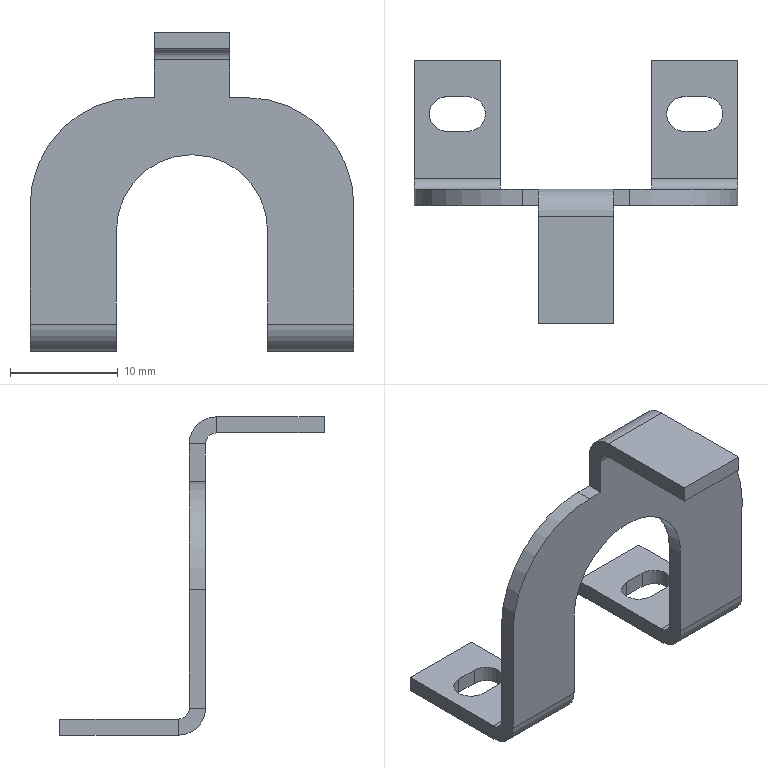Part | SolidWorks | features Fillet 3, ICE 3, EdgeFlange 2, Cut 1, FlatPattern 1, SMBaseFlange 1, SheetMetal 1 | 1 solid | 51 faces | box 30 x 24.5 x 29.5 mm | volume 1040 mm3 | plane 35 | cylinder 16 | commonest cylinder face diameters 3.2 x6 2 x3 5 x3 14 x2 20 x2
STEP:
#1=CARTESIAN_POINT('',(-1.685,53.528,-1.5));
#2=VERTEX_POINT('',#1);
#3=CARTESIAN_POINT('',(-0.08512,51.928,-1.5));
#4=VERTEX_POINT('',#3);
#5=CARTESIAN_POINT('',(-1.685,51.928,-1.5));
#6=DIRECTION('',(0.,0.,-1.));
#7=DIRECTION('',(-1.,0.,0.));
#8=AXIS2_PLACEMENT_3D('',#5,#6,#7);
#9=CIRCLE('',#8,1.6);
#10=EDGE_CURVE('',#2,#4,#9,.T.);
#11=ORIENTED_EDGE('',*,*,#10,.T.);
#12=CARTESIAN_POINT('',(-0.08512,51.928,0.));
#13=VERTEX_POINT('',#12);
#14=CARTESIAN_POINT('',(-0.08512,51.928,-10.));
#15=DIRECTION('',(0.,0.,1.));
#16=VECTOR('',#15,1000.);
#17=LINE('',#14,#16);
#18=EDGE_CURVE('',#4,#13,#17,.T.);
#19=ORIENTED_EDGE('',*,*,#18,.T.);
#20=CARTESIAN_POINT('',(-1.685,53.528,0.));
#21=VERTEX_POINT('',#20);
#22=CARTESIAN_POINT('',(-1.685,51.928,0.));
#23=DIRECTION('',(0.,0.,1.));
#24=DIRECTION('',(1.,0.,0.));
#25=AXIS2_PLACEMENT_3D('',#22,#23,#24);
#26=CIRCLE('',#25,1.6);
#27=EDGE_CURVE('',#13,#21,#26,.T.);
#28=ORIENTED_EDGE('',*,*,#27,.T.);
#29=CARTESIAN_POINT('',(-1.685,53.528,-10.));
#30=DIRECTION('',(0.,0.,1.));
#31=VECTOR('',#30,1000.);
#32=LINE('',#29,#31);
#33=EDGE_CURVE('',#2,#21,#32,.T.);
#34=ORIENTED_EDGE('',*,*,#33,.F.);
#35=EDGE_LOOP('',(#11,#19,#28,#34));
#36=FACE_OUTER_BOUND('',#35,.T.);
#37=CARTESIAN_POINT('',(-1.685,51.928,-10.));
#38=DIRECTION('',(0.,0.,1.));
#39=DIRECTION('',(1.,0.,0.));
#40=AXIS2_PLACEMENT_3D('',#37,#38,#39);
#41=CYLINDRICAL_SURFACE('',#40,1.6);
#42=ADVANCED_FACE('',(#36),#41,.F.);
#43=CARTESIAN_POINT('',(-23.685,53.528,-1.5));
#44=VERTEX_POINT('',#43);
#45=CARTESIAN_POINT('',(-22.085,51.928,-1.5));
#46=VERTEX_POINT('',#45);
#47=CARTESIAN_POINT('',(-23.685,51.928,-1.5));
#48=DIRECTION('',(0.,0.,-1.));
#49=DIRECTION('',(-1.,0.,0.));
#50=AXIS2_PLACEMENT_3D('',#47,#48,#49);
#51=CIRCLE('',#50,1.6);
#52=EDGE_CURVE('',#44,#46,#51,.T.);
#53=ORIENTED_EDGE('',*,*,#52,.T.);
#54=CARTESIAN_POINT('',(-22.085,51.928,0.));
#55=VERTEX_POINT('',#54);
#56=CARTESIAN_POINT('',(-22.085,51.928,-10.));
#57=DIRECTION('',(0.,0.,1.));
#58=VECTOR('',#57,1000.);
#59=LINE('',#56,#58);
#60=EDGE_CURVE('',#46,#55,#59,.T.);
#61=ORIENTED_EDGE('',*,*,#60,.T.);
#62=CARTESIAN_POINT('',(-23.685,53.528,0.));
#63=VERTEX_POINT('',#62);
#64=CARTESIAN_POINT('',(-23.685,51.928,0.));
#65=DIRECTION('',(0.,0.,1.));
#66=DIRECTION('',(1.,0.,0.));
#67=AXIS2_PLACEMENT_3D('',#64,#65,#66);
#68=CIRCLE('',#67,1.6);
#69=EDGE_CURVE('',#55,#63,#68,.T.);
#70=ORIENTED_EDGE('',*,*,#69,.T.);
#71=CARTESIAN_POINT('',(-23.685,53.528,-10.));
#72=DIRECTION('',(0.,0.,1.));
#73=VECTOR('',#72,1000.);
#74=LINE('',#71,#73);
#75=EDGE_CURVE('',#44,#63,#74,.T.);
#76=ORIENTED_EDGE('',*,*,#75,.F.);
#77=EDGE_LOOP('',(#53,#61,#70,#76));
#78=FACE_OUTER_BOUND('',#77,.T.);
#79=CARTESIAN_POINT('',(-23.685,51.928,-10.));
#80=DIRECTION('',(0.,0.,1.));
#81=DIRECTION('',(1.,0.,0.));
#82=AXIS2_PLACEMENT_3D('',#79,#80,#81);
#83=CYLINDRICAL_SURFACE('',#82,1.6);
#84=ADVANCED_FACE('',(#78),#83,.F.);
#85=CARTESIAN_POINT('',(-6.685,56.928,-1.5));
#86=VERTEX_POINT('',#85);
#87=CARTESIAN_POINT('',(-6.685,45.928,-1.5));
#88=VERTEX_POINT('',#87);
#89=CARTESIAN_POINT('',(-6.685,0.,-1.5));
#90=DIRECTION('',(0.,-1.,0.));
#91=VECTOR('',#90,1000.);
#92=LINE('',#89,#91);
#93=EDGE_CURVE('',#86,#88,#92,.T.);
#94=ORIENTED_EDGE('',*,*,#93,.T.);
#95=CARTESIAN_POINT('',(-6.685,45.928,0.));
#96=VERTEX_POINT('',#95);
#97=CARTESIAN_POINT('',(-6.685,45.928,-1.5));
#98=DIRECTION('',(0.,0.,1.));
#99=VECTOR('',#98,1000.);
#100=LINE('',#97,#99);
#101=EDGE_CURVE('',#88,#96,#100,.T.);
#102=ORIENTED_EDGE('',*,*,#101,.T.);
#103=CARTESIAN_POINT('',(-6.685,56.928,0.));
#104=VERTEX_POINT('',#103);
#105=CARTESIAN_POINT('',(-6.685,0.,0.));
#106=DIRECTION('',(0.,-1.,0.));
#107=VECTOR('',#106,1000.);
#108=LINE('',#105,#107);
#109=EDGE_CURVE('',#104,#96,#108,.T.);
#110=ORIENTED_EDGE('',*,*,#109,.F.);
#111=CARTESIAN_POINT('',(-6.685,56.928,-3.296));
#112=DIRECTION('',(0.,0.,-1.));
#113=VECTOR('',#112,1000.);
#114=LINE('',#111,#113);
#115=EDGE_CURVE('',#104,#86,#114,.T.);
#116=ORIENTED_EDGE('',*,*,#115,.T.);
#117=EDGE_LOOP('',(#94,#102,#110,#116));
#118=FACE_OUTER_BOUND('',#117,.T.);
#119=CARTESIAN_POINT('',(-6.685,32.427,-3.296));
#120=DIRECTION('',(1.,0.,0.));
#121=DIRECTION('',(0.,0.,-1.));
#122=AXIS2_PLACEMENT_3D('',#119,#120,#121);
#123=PLANE('',#122);
#124=ADVANCED_FACE('',(#118),#123,.F.);
#125=CARTESIAN_POINT('',(-6.685,43.428,9.704));
#126=VERTEX_POINT('',#125);
#127=CARTESIAN_POINT('',(-6.685,43.428,1.));
#128=VERTEX_POINT('',#127);
#129=CARTESIAN_POINT('',(-6.685,43.428,0.));
#130=DIRECTION('',(0.,0.,-1.));
#131=VECTOR('',#130,1000.);
#132=LINE('',#129,#131);
#133=EDGE_CURVE('',#126,#128,#132,.T.);
#134=ORIENTED_EDGE('',*,*,#133,.F.);
#135=CARTESIAN_POINT('',(-6.685,44.928,9.704));
#136=VERTEX_POINT('',#135);
#137=CARTESIAN_POINT('',(-6.685,44.928,9.704));
#138=DIRECTION('',(0.,1.,0.));
#139=VECTOR('',#138,1000.);
#140=LINE('',#137,#139);
#141=EDGE_CURVE('',#126,#136,#140,.T.);
#142=ORIENTED_EDGE('',*,*,#141,.T.);
#143=CARTESIAN_POINT('',(-6.685,44.928,1.));
#144=VERTEX_POINT('',#143);
#145=CARTESIAN_POINT('',(-6.685,44.928,0.));
#146=DIRECTION('',(0.,0.,-1.));
#147=VECTOR('',#146,1000.);
#148=LINE('',#145,#147);
#149=EDGE_CURVE('',#136,#144,#148,.T.);
#150=ORIENTED_EDGE('',*,*,#149,.T.);
#151=CARTESIAN_POINT('',(-6.685,44.928,1.));
#152=DIRECTION('',(0.,-1.,0.));
#153=VECTOR('',#152,1000.);
#154=LINE('',#151,#153);
#155=EDGE_CURVE('',#144,#128,#154,.T.);
#156=ORIENTED_EDGE('',*,*,#155,.T.);
#157=EDGE_LOOP('',(#134,#142,#150,#156));
#158=FACE_OUTER_BOUND('',#157,.T.);
#159=CARTESIAN_POINT('',(-6.685,32.427,-3.296));
#160=DIRECTION('',(1.,0.,0.));
#161=DIRECTION('',(0.,0.,-1.));
#162=AXIS2_PLACEMENT_3D('',#159,#160,#161);
#163=PLANE('',#162);
#164=ADVANCED_FACE('',(#158),#163,.F.);
#165=CARTESIAN_POINT('',(-20.685,45.928,0.));
#166=VERTEX_POINT('',#165);
#167=CARTESIAN_POINT('',(-20.685,56.928,0.));
#168=VERTEX_POINT('',#167);
#169=CARTESIAN_POINT('',(-20.685,0.,0.));
#170=DIRECTION('',(0.,1.,0.));
#171=VECTOR('',#170,1000.);
#172=LINE('',#169,#171);
#173=EDGE_CURVE('',#166,#168,#172,.T.);
#174=ORIENTED_EDGE('',*,*,#173,.F.);
#175=CARTESIAN_POINT('',(-20.685,45.928,-1.5));
#176=VERTEX_POINT('',#175);
#177=CARTESIAN_POINT('',(-20.685,45.928,0.));
#178=DIRECTION('',(0.,0.,-1.));
#179=VECTOR('',#178,1000.);
#180=LINE('',#177,#179);
#181=EDGE_CURVE('',#166,#176,#180,.T.);
#182=ORIENTED_EDGE('',*,*,#181,.T.);
#183=CARTESIAN_POINT('',(-20.685,56.928,-1.5));
#184=VERTEX_POINT('',#183);
#185=CARTESIAN_POINT('',(-20.685,0.,-1.5));
#186=DIRECTION('',(0.,1.,0.));
#187=VECTOR('',#186,1000.);
#188=LINE('',#185,#187);
#189=EDGE_CURVE('',#176,#184,#188,.T.);
#190=ORIENTED_EDGE('',*,*,#189,.T.);
#191=CARTESIAN_POINT('',(-20.685,56.928,-3.296));
#192=DIRECTION('',(0.,0.,1.));
#193=VECTOR('',#192,1000.);
#194=LINE('',#191,#193);
#195=EDGE_CURVE('',#184,#168,#194,.T.);
#196=ORIENTED_EDGE('',*,*,#195,.T.);
#197=EDGE_LOOP('',(#174,#182,#190,#196));
#198=FACE_OUTER_BOUND('',#197,.T.);
#199=CARTESIAN_POINT('',(-20.685,32.427,-3.296));
#200=DIRECTION('',(-1.,0.,0.));
#201=DIRECTION('',(0.,0.,1.));
#202=AXIS2_PLACEMENT_3D('',#199,#200,#201);
#203=PLANE('',#202);
#204=ADVANCED_FACE('',(#198),#203,.F.);
#205=CARTESIAN_POINT('',(-20.685,44.928,1.));
#206=VERTEX_POINT('',#205);
#207=CARTESIAN_POINT('',(-20.685,44.928,9.704));
#208=VERTEX_POINT('',#207);
#209=CARTESIAN_POINT('',(-20.685,44.928,0.));
#210=DIRECTION('',(0.,0.,1.));
#211=VECTOR('',#210,1000.);
#212=LINE('',#209,#211);
#213=EDGE_CURVE('',#206,#208,#212,.T.);
#214=ORIENTED_EDGE('',*,*,#213,.T.);
#215=CARTESIAN_POINT('',(-20.685,43.428,9.704));
#216=VERTEX_POINT('',#215);
#217=CARTESIAN_POINT('',(-20.685,43.428,9.704));
#218=DIRECTION('',(0.,-1.,0.));
#219=VECTOR('',#218,1000.);
#220=LINE('',#217,#219);
#221=EDGE_CURVE('',#208,#216,#220,.T.);
#222=ORIENTED_EDGE('',*,*,#221,.T.);
#223=CARTESIAN_POINT('',(-20.685,43.428,1.));
#224=VERTEX_POINT('',#223);
#225=CARTESIAN_POINT('',(-20.685,43.428,0.));
#226=DIRECTION('',(0.,0.,1.));
#227=VECTOR('',#226,1000.);
#228=LINE('',#225,#227);
#229=EDGE_CURVE('',#224,#216,#228,.T.);
#230=ORIENTED_EDGE('',*,*,#229,.F.);
#231=CARTESIAN_POINT('',(-20.685,43.428,1.));
#232=DIRECTION('',(0.,1.,0.));
#233=VECTOR('',#232,1000.);
#234=LINE('',#231,#233);
#235=EDGE_CURVE('',#224,#206,#234,.T.);
#236=ORIENTED_EDGE('',*,*,#235,.T.);
#237=EDGE_LOOP('',(#214,#222,#230,#236));
#238=FACE_OUTER_BOUND('',#237,.T.);
#239=CARTESIAN_POINT('',(-20.685,32.427,-3.296));
#240=DIRECTION('',(-1.,0.,0.));
#241=DIRECTION('',(0.,0.,1.));
#242=AXIS2_PLACEMENT_3D('',#239,#240,#241);
#243=PLANE('',#242);
#244=ADVANCED_FACE('',(#238),#243,.F.);
#245=CARTESIAN_POINT('',(-25.685,50.328,-1.5));
#246=VERTEX_POINT('',#245);
#247=CARTESIAN_POINT('',(-25.685,53.528,-1.5));
#248=VERTEX_POINT('',#247);
#249=CARTESIAN_POINT('',(-25.685,51.928,-1.5));
#250=DIRECTION('',(0.,0.,-1.));
#251=DIRECTION('',(-1.,0.,0.));
#252=AXIS2_PLACEMENT_3D('',#249,#250,#251);
#253=CIRCLE('',#252,1.6);
#254=EDGE_CURVE('',#246,#248,#253,.T.);
#255=ORIENTED_EDGE('',*,*,#254,.F.);
#256=CARTESIAN_POINT('',(-23.685,50.328,-1.5));
#257=VERTEX_POINT('',#256);
#258=CARTESIAN_POINT('',(0.,50.328,-1.5));
#259=DIRECTION('',(-1.,0.,0.));
#260=VECTOR('',#259,1000.);
#261=LINE('',#258,#260);
#262=EDGE_CURVE('',#257,#246,#261,.T.);
#263=ORIENTED_EDGE('',*,*,#262,.F.);
#264=CARTESIAN_POINT('',(-23.685,51.928,-1.5));
#265=DIRECTION('',(0.,0.,-1.));
#266=DIRECTION('',(-1.,0.,0.));
#267=AXIS2_PLACEMENT_3D('',#264,#265,#266);
#268=CIRCLE('',#267,1.6);
#269=EDGE_CURVE('',#46,#257,#268,.T.);
#270=ORIENTED_EDGE('',*,*,#269,.F.);
#271=ORIENTED_EDGE('',*,*,#52,.F.);
#272=CARTESIAN_POINT('',(0.,53.528,-1.5));
#273=DIRECTION('',(1.,0.,0.));
#274=VECTOR('',#273,1000.);
#275=LINE('',#272,#274);
#276=EDGE_CURVE('',#248,#44,#275,.T.);
#277=ORIENTED_EDGE('',*,*,#276,.F.);
#278=EDGE_LOOP('',(#255,#263,#270,#271,#277));
#279=FACE_BOUND('',#278,.T.);
#280=ORIENTED_EDGE('',*,*,#189,.F.);
#281=CARTESIAN_POINT('',(-28.685,45.928,-1.5));
#282=VERTEX_POINT('',#281);
#283=CARTESIAN_POINT('',(1.315,45.928,-1.5));
#284=DIRECTION('',(-1.,0.,0.));
#285=VECTOR('',#284,1000.);
#286=LINE('',#283,#285);
#287=EDGE_CURVE('',#176,#282,#286,.T.);
#288=ORIENTED_EDGE('',*,*,#287,.T.);
#289=CARTESIAN_POINT('',(-28.685,56.928,-1.5));
#290=VERTEX_POINT('',#289);
#291=CARTESIAN_POINT('',(-28.685,56.928,-1.5));
#292=DIRECTION('',(0.,-1.,0.));
#293=VECTOR('',#292,1000.);
#294=LINE('',#291,#293);
#295=EDGE_CURVE('',#290,#282,#294,.T.);
#296=ORIENTED_EDGE('',*,*,#295,.F.);
#297=CARTESIAN_POINT('',(1.315,56.928,-1.5));
#298=DIRECTION('',(-1.,0.,0.));
#299=VECTOR('',#298,1000.);
#300=LINE('',#297,#299);
#301=EDGE_CURVE('',#184,#290,#300,.T.);
#302=ORIENTED_EDGE('',*,*,#301,.F.);
#303=EDGE_LOOP('',(#280,#288,#296,#302));
#304=FACE_OUTER_BOUND('',#303,.T.);
#305=CARTESIAN_POINT('',(0.,0.,-1.5));
#306=DIRECTION('',(0.,0.,-1.));
#307=DIRECTION('',(-1.,0.,0.));
#308=AXIS2_PLACEMENT_3D('',#305,#306,#307);
#309=PLANE('',#308);
#310=ADVANCED_FACE('',(#279,#304),#309,.T.);
#311=CARTESIAN_POINT('',(-25.685,50.328,0.));
#312=VERTEX_POINT('',#311);
#313=CARTESIAN_POINT('',(-23.685,50.328,0.));
#314=VERTEX_POINT('',#313);
#315=CARTESIAN_POINT('',(-25.685,50.328,0.));
#316=DIRECTION('',(1.,0.,0.));
#317=VECTOR('',#316,1000.);
#318=LINE('',#315,#317);
#319=EDGE_CURVE('',#312,#314,#318,.T.);
#320=ORIENTED_EDGE('',*,*,#319,.F.);
#321=CARTESIAN_POINT('',(-25.685,53.528,0.));
#322=VERTEX_POINT('',#321);
#323=CARTESIAN_POINT('',(-25.685,51.928,0.));
#324=DIRECTION('',(0.,0.,1.));
#325=DIRECTION('',(1.,0.,0.));
#326=AXIS2_PLACEMENT_3D('',#323,#324,#325);
#327=CIRCLE('',#326,1.6);
#328=EDGE_CURVE('',#322,#312,#327,.T.);
#329=ORIENTED_EDGE('',*,*,#328,.F.);
#330=CARTESIAN_POINT('',(-25.685,53.528,0.));
#331=DIRECTION('',(-1.,0.,0.));
#332=VECTOR('',#331,1000.);
#333=LINE('',#330,#332);
#334=EDGE_CURVE('',#63,#322,#333,.T.);
#335=ORIENTED_EDGE('',*,*,#334,.F.);
#336=ORIENTED_EDGE('',*,*,#69,.F.);
#337=CARTESIAN_POINT('',(-23.685,51.928,0.));
#338=DIRECTION('',(0.,0.,1.));
#339=DIRECTION('',(1.,0.,0.));
#340=AXIS2_PLACEMENT_3D('',#337,#338,#339);
#341=CIRCLE('',#340,1.6);
#342=EDGE_CURVE('',#314,#55,#341,.T.);
#343=ORIENTED_EDGE('',*,*,#342,.F.);
#344=EDGE_LOOP('',(#320,#329,#335,#336,#343));
#345=FACE_BOUND('',#344,.T.);
#346=CARTESIAN_POINT('',(-28.685,45.928,0.));
#347=VERTEX_POINT('',#346);
#348=CARTESIAN_POINT('',(1.315,45.928,0.));
#349=DIRECTION('',(-1.,0.,0.));
#350=VECTOR('',#349,1000.);
#351=LINE('',#348,#350);
#352=EDGE_CURVE('',#166,#347,#351,.T.);
#353=ORIENTED_EDGE('',*,*,#352,.F.);
#354=ORIENTED_EDGE('',*,*,#173,.T.);
#355=CARTESIAN_POINT('',(-28.685,56.928,0.));
#356=VERTEX_POINT('',#355);
#357=CARTESIAN_POINT('',(1.315,56.928,0.));
#358=DIRECTION('',(-1.,0.,0.));
#359=VECTOR('',#358,1000.);
#360=LINE('',#357,#359);
#361=EDGE_CURVE('',#168,#356,#360,.T.);
#362=ORIENTED_EDGE('',*,*,#361,.T.);
#363=CARTESIAN_POINT('',(-28.685,56.928,0.));
#364=DIRECTION('',(0.,-1.,0.));
#365=VECTOR('',#364,1000.);
#366=LINE('',#363,#365);
#367=EDGE_CURVE('',#356,#347,#366,.T.);
#368=ORIENTED_EDGE('',*,*,#367,.T.);
#369=EDGE_LOOP('',(#353,#354,#362,#368));
#370=FACE_OUTER_BOUND('',#369,.T.);
#371=CARTESIAN_POINT('',(0.,0.,0.));
#372=DIRECTION('',(0.,0.,-1.));
#373=DIRECTION('',(-1.,0.,0.));
#374=AXIS2_PLACEMENT_3D('',#371,#372,#373);
#375=PLANE('',#374);
#376=ADVANCED_FACE('',(#345,#370),#375,.F.);
#377=ORIENTED_EDGE('',*,*,#195,.F.);
#378=ORIENTED_EDGE('',*,*,#301,.T.);
#379=CARTESIAN_POINT('',(-28.685,56.928,-1.5));
#380=DIRECTION('',(0.,0.,1.));
#381=VECTOR('',#380,1000.);
#382=LINE('',#379,#381);
#383=EDGE_CURVE('',#290,#356,#382,.T.);
#384=ORIENTED_EDGE('',*,*,#383,.T.);
#385=ORIENTED_EDGE('',*,*,#361,.F.);
#386=EDGE_LOOP('',(#377,#378,#384,#385));
#387=FACE_OUTER_BOUND('',#386,.T.);
#388=CARTESIAN_POINT('',(1.315,56.928,-1.5));
#389=DIRECTION('',(0.,1.,0.));
#390=DIRECTION('',(0.,0.,1.));
#391=AXIS2_PLACEMENT_3D('',#388,#389,#390);
#392=PLANE('',#391);
#393=ADVANCED_FACE('',(#387),#392,.T.);
#394=CARTESIAN_POINT('',(-20.685,45.928,1.));
#395=DIRECTION('',(1.,0.,0.));
#396=DIRECTION('',(0.,0.,1.));
#397=AXIS2_PLACEMENT_3D('',#394,#395,#396);
#398=CIRCLE('',#397,2.5);
#399=EDGE_CURVE('',#224,#176,#398,.T.);
#400=ORIENTED_EDGE('',*,*,#399,.F.);
#401=CARTESIAN_POINT('',(-28.685,43.428,1.));
#402=VERTEX_POINT('',#401);
#403=CARTESIAN_POINT('',(0.,43.428,1.));
#404=DIRECTION('',(-1.,0.,0.));
#405=VECTOR('',#404,1000.);
#406=LINE('',#403,#405);
#407=EDGE_CURVE('',#224,#402,#406,.T.);
#408=ORIENTED_EDGE('',*,*,#407,.T.);
#409=CARTESIAN_POINT('',(-28.685,45.928,1.));
#410=DIRECTION('',(-1.,0.,0.));
#411=DIRECTION('',(0.,0.,-1.));
#412=AXIS2_PLACEMENT_3D('',#409,#410,#411);
#413=CIRCLE('',#412,2.5);
#414=EDGE_CURVE('',#282,#402,#413,.T.);
#415=ORIENTED_EDGE('',*,*,#414,.F.);
#416=ORIENTED_EDGE('',*,*,#287,.F.);
#417=EDGE_LOOP('',(#400,#408,#415,#416));
#418=FACE_OUTER_BOUND('',#417,.T.);
#419=CARTESIAN_POINT('',(1.315,45.928,1.));
#420=DIRECTION('',(1.,0.,0.));
#421=DIRECTION('',(0.,-1.,0.));
#422=AXIS2_PLACEMENT_3D('',#419,#420,#421);
#423=CYLINDRICAL_SURFACE('',#422,2.5);
#424=ADVANCED_FACE('',(#418),#423,.T.);
#425=CARTESIAN_POINT('',(-28.685,44.928,1.));
#426=VERTEX_POINT('',#425);
#427=CARTESIAN_POINT('',(-28.685,44.928,1.));
#428=DIRECTION('',(1.,0.,0.));
#429=VECTOR('',#428,1000.);
#430=LINE('',#427,#429);
#431=EDGE_CURVE('',#426,#206,#430,.T.);
#432=ORIENTED_EDGE('',*,*,#431,.T.);
#433=CARTESIAN_POINT('',(-20.685,45.928,1.));
#434=DIRECTION('',(1.,0.,0.));
#435=DIRECTION('',(0.,0.,1.));
#436=AXIS2_PLACEMENT_3D('',#433,#434,#435);
#437=CIRCLE('',#436,1.);
#438=EDGE_CURVE('',#206,#166,#437,.T.);
#439=ORIENTED_EDGE('',*,*,#438,.T.);
#440=ORIENTED_EDGE('',*,*,#352,.T.);
#441=CARTESIAN_POINT('',(-28.685,45.928,1.));
#442=DIRECTION('',(-1.,0.,0.));
#443=DIRECTION('',(0.,0.,-1.));
#444=AXIS2_PLACEMENT_3D('',#441,#442,#443);
#445=CIRCLE('',#444,1.);
#446=EDGE_CURVE('',#347,#426,#445,.T.);
#447=ORIENTED_EDGE('',*,*,#446,.T.);
#448=EDGE_LOOP('',(#432,#439,#440,#447));
#449=FACE_OUTER_BOUND('',#448,.T.);
#450=CARTESIAN_POINT('',(1.315,45.928,1.));
#451=DIRECTION('',(1.,0.,0.));
#452=DIRECTION('',(0.,-1.,0.));
#453=AXIS2_PLACEMENT_3D('',#450,#451,#452);
#454=CYLINDRICAL_SURFACE('',#453,1.);
#455=ADVANCED_FACE('',(#449),#454,.F.);
#456=CARTESIAN_POINT('',(1.315,43.428,1.));
#457=VERTEX_POINT('',#456);
#458=CARTESIAN_POINT('',(1.315,43.428,12.));
#459=VERTEX_POINT('',#458);
#460=CARTESIAN_POINT('',(1.315,43.427,26.5));
#461=DIRECTION('',(0.,0.,1.));
#462=VECTOR('',#461,1000.);
#463=LINE('',#460,#462);
#464=EDGE_CURVE('',#457,#459,#463,.T.);
#465=ORIENTED_EDGE('',*,*,#464,.T.);
#466=CARTESIAN_POINT('',(-8.685,43.428,22.));
#467=VERTEX_POINT('',#466);
#468=CARTESIAN_POINT('',(-8.685,43.428,12.));
#469=DIRECTION('',(0.,-1.,0.));
#470=DIRECTION('',(0.,0.,1.));
#471=AXIS2_PLACEMENT_3D('',#468,#469,#470);
#472=CIRCLE('',#471,10.);
#473=EDGE_CURVE('',#459,#467,#472,.T.);
#474=ORIENTED_EDGE('',*,*,#473,.T.);
#475=CARTESIAN_POINT('',(-10.185,43.428,22.));
#476=VERTEX_POINT('',#475);
#477=CARTESIAN_POINT('',(0.,43.428,22.));
#478=DIRECTION('',(1.,0.,0.));
#479=VECTOR('',#478,1000.);
#480=LINE('',#477,#479);
#481=EDGE_CURVE('',#476,#467,#480,.T.);
#482=ORIENTED_EDGE('',*,*,#481,.F.);
#483=CARTESIAN_POINT('',(-10.185,43.427,25.5));
#484=VERTEX_POINT('',#483);
#485=CARTESIAN_POINT('',(-10.185,43.428,0.));
#486=DIRECTION('',(0.,0.,1.));
#487=VECTOR('',#486,1000.);
#488=LINE('',#485,#487);
#489=EDGE_CURVE('',#476,#484,#488,.T.);
#490=ORIENTED_EDGE('',*,*,#489,.T.);
#491=CARTESIAN_POINT('',(-17.185,43.427,25.5));
#492=VERTEX_POINT('',#491);
#493=CARTESIAN_POINT('',(-28.685,43.427,25.5));
#494=DIRECTION('',(1.,0.,0.));
#495=VECTOR('',#494,1000.);
#496=LINE('',#493,#495);
#497=EDGE_CURVE('',#492,#484,#496,.T.);
#498=ORIENTED_EDGE('',*,*,#497,.F.);
#499=CARTESIAN_POINT('',(-17.185,43.427,22.));
#500=VERTEX_POINT('',#499);
#501=CARTESIAN_POINT('',(-17.185,43.428,0.));
#502=DIRECTION('',(0.,0.,-1.));
#503=VECTOR('',#502,1000.);
#504=LINE('',#501,#503);
#505=EDGE_CURVE('',#492,#500,#504,.T.);
#506=ORIENTED_EDGE('',*,*,#505,.T.);
#507=CARTESIAN_POINT('',(-18.685,43.427,22.));
#508=VERTEX_POINT('',#507);
#509=CARTESIAN_POINT('',(0.,43.428,22.));
#510=DIRECTION('',(-1.,0.,0.));
#511=VECTOR('',#510,1000.);
#512=LINE('',#509,#511);
#513=EDGE_CURVE('',#500,#508,#512,.T.);
#514=ORIENTED_EDGE('',*,*,#513,.T.);
#515=CARTESIAN_POINT('',(-28.685,43.428,12.));
#516=VERTEX_POINT('',#515);
#517=CARTESIAN_POINT('',(-18.685,43.428,12.));
#518=DIRECTION('',(0.,-1.,0.));
#519=DIRECTION('',(0.,0.,1.));
#520=AXIS2_PLACEMENT_3D('',#517,#518,#519);
#521=CIRCLE('',#520,10.);
#522=EDGE_CURVE('',#508,#516,#521,.T.);
#523=ORIENTED_EDGE('',*,*,#522,.T.);
#524=CARTESIAN_POINT('',(-28.685,43.428,0.));
#525=DIRECTION('',(0.,0.,-1.));
#526=VECTOR('',#525,1000.);
#527=LINE('',#524,#526);
#528=EDGE_CURVE('',#516,#402,#527,.T.);
#529=ORIENTED_EDGE('',*,*,#528,.T.);
#530=ORIENTED_EDGE('',*,*,#407,.F.);
#531=ORIENTED_EDGE('',*,*,#229,.T.);
#532=CARTESIAN_POINT('',(-13.685,43.428,16.704));
#533=VERTEX_POINT('',#532);
#534=CARTESIAN_POINT('',(-13.685,43.428,9.704));
#535=DIRECTION('',(0.,1.,0.));
#536=DIRECTION('',(0.,0.,1.));
#537=AXIS2_PLACEMENT_3D('',#534,#535,#536);
#538=CIRCLE('',#537,7.);
#539=EDGE_CURVE('',#216,#533,#538,.T.);
#540=ORIENTED_EDGE('',*,*,#539,.T.);
#541=CARTESIAN_POINT('',(-13.685,43.428,9.704));
#542=DIRECTION('',(0.,1.,0.));
#543=DIRECTION('',(0.,0.,1.));
#544=AXIS2_PLACEMENT_3D('',#541,#542,#543);
#545=CIRCLE('',#544,7.);
#546=EDGE_CURVE('',#533,#126,#545,.T.);
#547=ORIENTED_EDGE('',*,*,#546,.T.);
#548=ORIENTED_EDGE('',*,*,#133,.T.);
#549=CARTESIAN_POINT('',(0.,43.428,1.));
#550=DIRECTION('',(-1.,0.,0.));
#551=VECTOR('',#550,1000.);
#552=LINE('',#549,#551);
#553=EDGE_CURVE('',#457,#128,#552,.T.);
#554=ORIENTED_EDGE('',*,*,#553,.F.);
#555=EDGE_LOOP('',(#465,#474,#482,#490,#498,#506,#514,#523,#529,#530,#531,#540,#547,#548,#554));
#556=FACE_OUTER_BOUND('',#555,.T.);
#557=CARTESIAN_POINT('',(0.,43.428,0.));
#558=DIRECTION('',(0.,1.,0.));
#559=DIRECTION('',(0.,0.,1.));
#560=AXIS2_PLACEMENT_3D('',#557,#558,#559);
#561=PLANE('',#560);
#562=ADVANCED_FACE('',(#556),#561,.F.);
#563=CARTESIAN_POINT('',(-10.185,44.928,22.));
#564=VERTEX_POINT('',#563);
#565=CARTESIAN_POINT('',(-8.685,44.928,22.));
#566=VERTEX_POINT('',#565);
#567=CARTESIAN_POINT('',(0.,44.928,22.));
#568=DIRECTION('',(1.,0.,0.));
#569=VECTOR('',#568,1000.);
#570=LINE('',#567,#569);
#571=EDGE_CURVE('',#564,#566,#570,.T.);
#572=ORIENTED_EDGE('',*,*,#571,.T.);
#573=CARTESIAN_POINT('',(1.315,44.928,12.));
#574=VERTEX_POINT('',#573);
#575=CARTESIAN_POINT('',(-8.685,44.928,12.));
#576=DIRECTION('',(0.,1.,0.));
#577=DIRECTION('',(0.,0.,1.));
#578=AXIS2_PLACEMENT_3D('',#575,#576,#577);
#579=CIRCLE('',#578,10.);
#580=EDGE_CURVE('',#566,#574,#579,.T.);
#581=ORIENTED_EDGE('',*,*,#580,.T.);
#582=CARTESIAN_POINT('',(1.315,44.928,1.));
#583=VERTEX_POINT('',#582);
#584=CARTESIAN_POINT('',(1.315,44.927,26.5));
#585=DIRECTION('',(0.,0.,1.));
#586=VECTOR('',#585,1000.);
#587=LINE('',#584,#586);
#588=EDGE_CURVE('',#583,#574,#587,.T.);
#589=ORIENTED_EDGE('',*,*,#588,.F.);
#590=CARTESIAN_POINT('',(-28.685,44.928,1.));
#591=DIRECTION('',(1.,0.,0.));
#592=VECTOR('',#591,1000.);
#593=LINE('',#590,#592);
#594=EDGE_CURVE('',#144,#583,#593,.T.);
#595=ORIENTED_EDGE('',*,*,#594,.F.);
#596=ORIENTED_EDGE('',*,*,#149,.F.);
#597=CARTESIAN_POINT('',(-13.685,44.928,16.704));
#598=VERTEX_POINT('',#597);
#599=CARTESIAN_POINT('',(-13.685,44.928,9.704));
#600=DIRECTION('',(0.,-1.,0.));
#601=DIRECTION('',(0.,0.,1.));
#602=AXIS2_PLACEMENT_3D('',#599,#600,#601);
#603=CIRCLE('',#602,7.);
#604=EDGE_CURVE('',#136,#598,#603,.T.);
#605=ORIENTED_EDGE('',*,*,#604,.T.);
#606=CARTESIAN_POINT('',(-13.685,44.928,9.704));
#607=DIRECTION('',(0.,-1.,0.));
#608=DIRECTION('',(0.,0.,1.));
#609=AXIS2_PLACEMENT_3D('',#606,#607,#608);
#610=CIRCLE('',#609,7.);
#611=EDGE_CURVE('',#598,#208,#610,.T.);
#612=ORIENTED_EDGE('',*,*,#611,.T.);
#613=ORIENTED_EDGE('',*,*,#213,.F.);
#614=ORIENTED_EDGE('',*,*,#431,.F.);
#615=CARTESIAN_POINT('',(-28.685,44.928,12.));
#616=VERTEX_POINT('',#615);
#617=CARTESIAN_POINT('',(-28.685,44.928,0.));
#618=DIRECTION('',(0.,0.,-1.));
#619=VECTOR('',#618,1000.);
#620=LINE('',#617,#619);
#621=EDGE_CURVE('',#616,#426,#620,.T.);
#622=ORIENTED_EDGE('',*,*,#621,.F.);
#623=CARTESIAN_POINT('',(-18.685,44.927,22.));
#624=VERTEX_POINT('',#623);
#625=CARTESIAN_POINT('',(-18.685,44.928,12.));
#626=DIRECTION('',(0.,1.,0.));
#627=DIRECTION('',(0.,0.,1.));
#628=AXIS2_PLACEMENT_3D('',#625,#626,#627);
#629=CIRCLE('',#628,10.);
#630=EDGE_CURVE('',#616,#624,#629,.T.);
#631=ORIENTED_EDGE('',*,*,#630,.T.);
#632=CARTESIAN_POINT('',(-17.185,44.927,22.));
#633=VERTEX_POINT('',#632);
#634=CARTESIAN_POINT('',(0.,44.928,22.));
#635=DIRECTION('',(-1.,0.,0.));
#636=VECTOR('',#635,1000.);
#637=LINE('',#634,#636);
#638=EDGE_CURVE('',#633,#624,#637,.T.);
#639=ORIENTED_EDGE('',*,*,#638,.F.);
#640=CARTESIAN_POINT('',(-17.185,44.927,25.5));
#641=VERTEX_POINT('',#640);
#642=CARTESIAN_POINT('',(-17.185,44.928,0.));
#643=DIRECTION('',(0.,0.,-1.));
#644=VECTOR('',#643,1000.);
#645=LINE('',#642,#644);
#646=EDGE_CURVE('',#641,#633,#645,.T.);
#647=ORIENTED_EDGE('',*,*,#646,.F.);
#648=CARTESIAN_POINT('',(-10.185,44.927,25.5));
#649=VERTEX_POINT('',#648);
#650=CARTESIAN_POINT('',(-28.685,44.927,25.5));
#651=DIRECTION('',(1.,0.,0.));
#652=VECTOR('',#651,1000.);
#653=LINE('',#650,#652);
#654=EDGE_CURVE('',#641,#649,#653,.T.);
#655=ORIENTED_EDGE('',*,*,#654,.T.);
#656=CARTESIAN_POINT('',(-10.185,44.928,0.));
#657=DIRECTION('',(0.,0.,1.));
#658=VECTOR('',#657,1000.);
#659=LINE('',#656,#658);
#660=EDGE_CURVE('',#564,#649,#659,.T.);
#661=ORIENTED_EDGE('',*,*,#660,.F.);
#662=EDGE_LOOP('',(#572,#581,#589,#595,#596,#605,#612,#613,#614,#622,#631,#639,#647,#655,#661));
#663=FACE_OUTER_BOUND('',#662,.T.);
#664=CARTESIAN_POINT('',(0.,44.928,0.));
#665=DIRECTION('',(0.,1.,0.));
#666=DIRECTION('',(0.,0.,1.));
#667=AXIS2_PLACEMENT_3D('',#664,#665,#666);
#668=PLANE('',#667);
#669=ADVANCED_FACE('',(#663),#668,.T.);
#670=CARTESIAN_POINT('',(-17.185,42.427,28.));
#671=VERTEX_POINT('',#670);
#672=CARTESIAN_POINT('',(-10.185,42.427,28.));
#673=VERTEX_POINT('',#672);
#674=CARTESIAN_POINT('',(0.,42.427,28.));
#675=DIRECTION('',(1.,0.,0.));
#676=VECTOR('',#675,1000.);
#677=LINE('',#674,#676);
#678=EDGE_CURVE('',#671,#673,#677,.T.);
#679=ORIENTED_EDGE('',*,*,#678,.T.);
#680=CARTESIAN_POINT('',(-10.185,42.427,25.5));
#681=DIRECTION('',(1.,0.,0.));
#682=DIRECTION('',(0.,0.,1.));
#683=AXIS2_PLACEMENT_3D('',#680,#681,#682);
#684=CIRCLE('',#683,2.5);
#685=EDGE_CURVE('',#649,#673,#684,.T.);
#686=ORIENTED_EDGE('',*,*,#685,.F.);
#687=ORIENTED_EDGE('',*,*,#654,.F.);
#688=CARTESIAN_POINT('',(-17.185,42.427,25.5));
#689=DIRECTION('',(-1.,0.,0.));
#690=DIRECTION('',(0.,0.,-1.));
#691=AXIS2_PLACEMENT_3D('',#688,#689,#690);
#692=CIRCLE('',#691,2.5);
#693=EDGE_CURVE('',#671,#641,#692,.T.);
#694=ORIENTED_EDGE('',*,*,#693,.F.);
#695=EDGE_LOOP('',(#679,#686,#687,#694));
#696=FACE_OUTER_BOUND('',#695,.T.);
#697=CARTESIAN_POINT('',(-28.685,42.427,25.5));
#698=DIRECTION('',(-1.,0.,0.));
#699=DIRECTION('',(0.,0.,1.));
#700=AXIS2_PLACEMENT_3D('',#697,#698,#699);
#701=CYLINDRICAL_SURFACE('',#700,2.5);
#702=ADVANCED_FACE('',(#696),#701,.T.);
#703=CARTESIAN_POINT('',(-10.185,42.427,26.5));
#704=VERTEX_POINT('',#703);
#705=CARTESIAN_POINT('',(-10.185,42.427,25.5));
#706=DIRECTION('',(1.,0.,0.));
#707=DIRECTION('',(0.,0.,1.));
#708=AXIS2_PLACEMENT_3D('',#705,#706,#707);
#709=CIRCLE('',#708,1.);
#710=EDGE_CURVE('',#484,#704,#709,.T.);
#711=ORIENTED_EDGE('',*,*,#710,.T.);
#712=CARTESIAN_POINT('',(-17.185,42.427,26.5));
#713=VERTEX_POINT('',#712);
#714=CARTESIAN_POINT('',(1.315,42.427,26.5));
#715=DIRECTION('',(-1.,0.,0.));
#716=VECTOR('',#715,1000.);
#717=LINE('',#714,#716);
#718=EDGE_CURVE('',#704,#713,#717,.T.);
#719=ORIENTED_EDGE('',*,*,#718,.T.);
#720=CARTESIAN_POINT('',(-17.185,42.427,25.5));
#721=DIRECTION('',(-1.,0.,0.));
#722=DIRECTION('',(0.,0.,1.));
#723=AXIS2_PLACEMENT_3D('',#720,#721,#722);
#724=CIRCLE('',#723,1.);
#725=EDGE_CURVE('',#713,#492,#724,.T.);
#726=ORIENTED_EDGE('',*,*,#725,.T.);
#727=ORIENTED_EDGE('',*,*,#497,.T.);
#728=EDGE_LOOP('',(#711,#719,#726,#727));
#729=FACE_OUTER_BOUND('',#728,.T.);
#730=CARTESIAN_POINT('',(-28.685,42.427,25.5));
#731=DIRECTION('',(-1.,0.,0.));
#732=DIRECTION('',(0.,0.,1.));
#733=AXIS2_PLACEMENT_3D('',#730,#731,#732);
#734=CYLINDRICAL_SURFACE('',#733,1.);
#735=ADVANCED_FACE('',(#729),#734,.F.);
#736=CARTESIAN_POINT('',(-10.185,32.427,28.));
#737=VERTEX_POINT('',#736);
#738=CARTESIAN_POINT('',(-10.185,0.,28.));
#739=DIRECTION('',(0.,1.,0.));
#740=VECTOR('',#739,1000.);
#741=LINE('',#738,#740);
#742=EDGE_CURVE('',#737,#673,#741,.T.);
#743=ORIENTED_EDGE('',*,*,#742,.T.);
#744=ORIENTED_EDGE('',*,*,#678,.F.);
#745=CARTESIAN_POINT('',(-17.185,32.427,28.));
#746=VERTEX_POINT('',#745);
#747=CARTESIAN_POINT('',(-17.185,32.427,28.));
#748=DIRECTION('',(0.,1.,0.));
#749=VECTOR('',#748,1000.);
#750=LINE('',#747,#749);
#751=EDGE_CURVE('',#746,#671,#750,.T.);
#752=ORIENTED_EDGE('',*,*,#751,.F.);
#753=CARTESIAN_POINT('',(1.315,32.427,28.));
#754=DIRECTION('',(1.,0.,0.));
#755=VECTOR('',#754,1000.);
#756=LINE('',#753,#755);
#757=EDGE_CURVE('',#746,#737,#756,.T.);
#758=ORIENTED_EDGE('',*,*,#757,.T.);
#759=EDGE_LOOP('',(#743,#744,#752,#758));
#760=FACE_OUTER_BOUND('',#759,.T.);
#761=CARTESIAN_POINT('',(0.,0.,28.));
#762=DIRECTION('',(0.,0.,-1.));
#763=DIRECTION('',(-1.,0.,0.));
#764=AXIS2_PLACEMENT_3D('',#761,#762,#763);
#765=PLANE('',#764);
#766=ADVANCED_FACE('',(#760),#765,.F.);
#767=ORIENTED_EDGE('',*,*,#718,.F.);
#768=CARTESIAN_POINT('',(-10.185,32.427,26.5));
#769=VERTEX_POINT('',#768);
#770=CARTESIAN_POINT('',(-10.185,0.,26.5));
#771=DIRECTION('',(0.,1.,0.));
#772=VECTOR('',#771,1000.);
#773=LINE('',#770,#772);
#774=EDGE_CURVE('',#769,#704,#773,.T.);
#775=ORIENTED_EDGE('',*,*,#774,.F.);
#776=CARTESIAN_POINT('',(-17.185,32.427,26.5));
#777=VERTEX_POINT('',#776);
#778=CARTESIAN_POINT('',(1.315,32.427,26.5));
#779=DIRECTION('',(1.,0.,0.));
#780=VECTOR('',#779,1000.);
#781=LINE('',#778,#780);
#782=EDGE_CURVE('',#777,#769,#781,.T.);
#783=ORIENTED_EDGE('',*,*,#782,.F.);
#784=CARTESIAN_POINT('',(-17.185,0.,26.5));
#785=DIRECTION('',(0.,1.,0.));
#786=VECTOR('',#785,1000.);
#787=LINE('',#784,#786);
#788=EDGE_CURVE('',#777,#713,#787,.T.);
#789=ORIENTED_EDGE('',*,*,#788,.T.);
#790=EDGE_LOOP('',(#767,#775,#783,#789));
#791=FACE_OUTER_BOUND('',#790,.T.);
#792=CARTESIAN_POINT('',(0.,0.,26.5));
#793=DIRECTION('',(0.,0.,-1.));
#794=DIRECTION('',(-1.,0.,0.));
#795=AXIS2_PLACEMENT_3D('',#792,#793,#794);
#796=PLANE('',#795);
#797=ADVANCED_FACE('',(#791),#796,.T.);
#798=CARTESIAN_POINT('',(-10.185,32.427,26.5));
#799=DIRECTION('',(0.,0.,1.));
#800=VECTOR('',#799,1000.);
#801=LINE('',#798,#800);
#802=EDGE_CURVE('',#769,#737,#801,.T.);
#803=ORIENTED_EDGE('',*,*,#802,.T.);
#804=ORIENTED_EDGE('',*,*,#757,.F.);
#805=CARTESIAN_POINT('',(-17.185,32.427,28.));
#806=DIRECTION('',(0.,0.,-1.));
#807=VECTOR('',#806,1000.);
#808=LINE('',#805,#807);
#809=EDGE_CURVE('',#746,#777,#808,.T.);
#810=ORIENTED_EDGE('',*,*,#809,.T.);
#811=ORIENTED_EDGE('',*,*,#782,.T.);
#812=EDGE_LOOP('',(#803,#804,#810,#811));
#813=FACE_OUTER_BOUND('',#812,.T.);
#814=CARTESIAN_POINT('',(1.315,32.427,28.));
#815=DIRECTION('',(0.,1.,0.));
#816=DIRECTION('',(0.,0.,1.));
#817=AXIS2_PLACEMENT_3D('',#814,#815,#816);
#818=PLANE('',#817);
#819=ADVANCED_FACE('',(#813),#818,.F.);
#820=ORIENTED_EDGE('',*,*,#588,.T.);
#821=CARTESIAN_POINT('',(1.315,43.428,12.));
#822=DIRECTION('',(0.,-1.,0.));
#823=VECTOR('',#822,1000.);
#824=LINE('',#821,#823);
#825=EDGE_CURVE('',#574,#459,#824,.T.);
#826=ORIENTED_EDGE('',*,*,#825,.T.);
#827=ORIENTED_EDGE('',*,*,#464,.F.);
#828=CARTESIAN_POINT('',(1.315,44.928,1.));
#829=DIRECTION('',(0.,-1.,0.));
#830=VECTOR('',#829,1000.);
#831=LINE('',#828,#830);
#832=EDGE_CURVE('',#583,#457,#831,.T.);
#833=ORIENTED_EDGE('',*,*,#832,.F.);
#834=EDGE_LOOP('',(#820,#826,#827,#833));
#835=FACE_OUTER_BOUND('',#834,.T.);
#836=CARTESIAN_POINT('',(1.315,43.427,26.5));
#837=DIRECTION('',(-1.,0.,0.));
#838=DIRECTION('',(0.,0.,1.));
#839=AXIS2_PLACEMENT_3D('',#836,#837,#838);
#840=PLANE('',#839);
#841=ADVANCED_FACE('',(#835),#840,.F.);
#842=ORIENTED_EDGE('',*,*,#528,.F.);
#843=CARTESIAN_POINT('',(-28.685,44.928,12.));
#844=DIRECTION('',(0.,1.,0.));
#845=VECTOR('',#844,1000.);
#846=LINE('',#843,#845);
#847=EDGE_CURVE('',#516,#616,#846,.T.);
#848=ORIENTED_EDGE('',*,*,#847,.T.);
#849=ORIENTED_EDGE('',*,*,#621,.T.);
#850=CARTESIAN_POINT('',(-28.685,44.928,1.));
#851=DIRECTION('',(0.,-1.,0.));
#852=VECTOR('',#851,1000.);
#853=LINE('',#850,#852);
#854=EDGE_CURVE('',#426,#402,#853,.T.);
#855=ORIENTED_EDGE('',*,*,#854,.T.);
#856=EDGE_LOOP('',(#842,#848,#849,#855));
#857=FACE_OUTER_BOUND('',#856,.T.);
#858=CARTESIAN_POINT('',(-28.685,43.428,0.));
#859=DIRECTION('',(1.,0.,0.));
#860=DIRECTION('',(0.,1.,0.));
#861=AXIS2_PLACEMENT_3D('',#858,#859,#860);
#862=PLANE('',#861);
#863=ADVANCED_FACE('',(#857),#862,.F.);
#864=CARTESIAN_POINT('',(1.315,45.928,0.));
#865=VERTEX_POINT('',#864);
#866=CARTESIAN_POINT('',(1.315,56.928,0.));
#867=VERTEX_POINT('',#866);
#868=CARTESIAN_POINT('',(1.315,56.928,0.));
#869=DIRECTION('',(0.,1.,0.));
#870=VECTOR('',#869,1000.);
#871=LINE('',#868,#870);
#872=EDGE_CURVE('',#865,#867,#871,.T.);
#873=ORIENTED_EDGE('',*,*,#872,.F.);
#874=CARTESIAN_POINT('',(1.315,45.928,-1.5));
#875=VERTEX_POINT('',#874);
#876=CARTESIAN_POINT('',(1.315,45.928,0.));
#877=DIRECTION('',(0.,0.,-1.));
#878=VECTOR('',#877,1000.);
#879=LINE('',#876,#878);
#880=EDGE_CURVE('',#865,#875,#879,.T.);
#881=ORIENTED_EDGE('',*,*,#880,.T.);
#882=CARTESIAN_POINT('',(1.315,56.928,-1.5));
#883=VERTEX_POINT('',#882);
#884=CARTESIAN_POINT('',(1.315,56.928,-1.5));
#885=DIRECTION('',(0.,1.,0.));
#886=VECTOR('',#885,1000.);
#887=LINE('',#884,#886);
#888=EDGE_CURVE('',#875,#883,#887,.T.);
#889=ORIENTED_EDGE('',*,*,#888,.T.);
#890=CARTESIAN_POINT('',(1.315,56.928,-1.5));
#891=DIRECTION('',(0.,0.,1.));
#892=VECTOR('',#891,1000.);
#893=LINE('',#890,#892);
#894=EDGE_CURVE('',#883,#867,#893,.T.);
#895=ORIENTED_EDGE('',*,*,#894,.T.);
#896=EDGE_LOOP('',(#873,#881,#889,#895));
#897=FACE_OUTER_BOUND('',#896,.T.);
#898=CARTESIAN_POINT('',(1.315,56.928,-1.5));
#899=DIRECTION('',(1.,0.,0.));
#900=DIRECTION('',(0.,1.,0.));
#901=AXIS2_PLACEMENT_3D('',#898,#899,#900);
#902=PLANE('',#901);
#903=ADVANCED_FACE('',(#897),#902,.T.);
#904=CARTESIAN_POINT('',(-3.685,50.328,-1.5));
#905=VERTEX_POINT('',#904);
#906=CARTESIAN_POINT('',(-3.685,53.528,-1.5));
#907=VERTEX_POINT('',#906);
#908=CARTESIAN_POINT('',(-3.685,51.928,-1.5));
#909=DIRECTION('',(0.,0.,-1.));
#910=DIRECTION('',(-1.,0.,0.));
#911=AXIS2_PLACEMENT_3D('',#908,#909,#910);
#912=CIRCLE('',#911,1.6);
#913=EDGE_CURVE('',#905,#907,#912,.T.);
#914=ORIENTED_EDGE('',*,*,#913,.F.);
#915=CARTESIAN_POINT('',(-1.685,50.328,-1.5));
#916=VERTEX_POINT('',#915);
#917=CARTESIAN_POINT('',(0.,50.328,-1.5));
#918=DIRECTION('',(-1.,0.,0.));
#919=VECTOR('',#918,1000.);
#920=LINE('',#917,#919);
#921=EDGE_CURVE('',#916,#905,#920,.T.);
#922=ORIENTED_EDGE('',*,*,#921,.F.);
#923=CARTESIAN_POINT('',(-1.685,51.928,-1.5));
#924=DIRECTION('',(0.,0.,-1.));
#925=DIRECTION('',(-1.,0.,0.));
#926=AXIS2_PLACEMENT_3D('',#923,#924,#925);
#927=CIRCLE('',#926,1.6);
#928=EDGE_CURVE('',#4,#916,#927,.T.);
#929=ORIENTED_EDGE('',*,*,#928,.F.);
#930=ORIENTED_EDGE('',*,*,#10,.F.);
#931=CARTESIAN_POINT('',(0.,53.528,-1.5));
#932=DIRECTION('',(1.,0.,0.));
#933=VECTOR('',#932,1000.);
#934=LINE('',#931,#933);
#935=EDGE_CURVE('',#907,#2,#934,.T.);
#936=ORIENTED_EDGE('',*,*,#935,.F.);
#937=EDGE_LOOP('',(#914,#922,#929,#930,#936));
#938=FACE_BOUND('',#937,.T.);
#939=ORIENTED_EDGE('',*,*,#93,.F.);
#940=CARTESIAN_POINT('',(1.315,56.928,-1.5));
#941=DIRECTION('',(-1.,0.,0.));
#942=VECTOR('',#941,1000.);
#943=LINE('',#940,#942);
#944=EDGE_CURVE('',#883,#86,#943,.T.);
#945=ORIENTED_EDGE('',*,*,#944,.F.);
#946=ORIENTED_EDGE('',*,*,#888,.F.);
#947=CARTESIAN_POINT('',(1.315,45.928,-1.5));
#948=DIRECTION('',(-1.,0.,0.));
#949=VECTOR('',#948,1000.);
#950=LINE('',#947,#949);
#951=EDGE_CURVE('',#875,#88,#950,.T.);
#952=ORIENTED_EDGE('',*,*,#951,.T.);
#953=EDGE_LOOP('',(#939,#945,#946,#952));
#954=FACE_OUTER_BOUND('',#953,.T.);
#955=CARTESIAN_POINT('',(0.,0.,-1.5));
#956=DIRECTION('',(0.,0.,-1.));
#957=DIRECTION('',(-1.,0.,0.));
#958=AXIS2_PLACEMENT_3D('',#955,#956,#957);
#959=PLANE('',#958);
#960=ADVANCED_FACE('',(#938,#954),#959,.T.);
#961=CARTESIAN_POINT('',(-3.685,50.328,0.));
#962=VERTEX_POINT('',#961);
#963=CARTESIAN_POINT('',(-1.685,50.328,0.));
#964=VERTEX_POINT('',#963);
#965=CARTESIAN_POINT('',(-3.685,50.328,0.));
#966=DIRECTION('',(1.,0.,0.));
#967=VECTOR('',#966,1000.);
#968=LINE('',#965,#967);
#969=EDGE_CURVE('',#962,#964,#968,.T.);
#970=ORIENTED_EDGE('',*,*,#969,.F.);
#971=CARTESIAN_POINT('',(-3.685,53.528,0.));
#972=VERTEX_POINT('',#971);
#973=CARTESIAN_POINT('',(-3.685,51.928,0.));
#974=DIRECTION('',(0.,0.,1.));
#975=DIRECTION('',(1.,0.,0.));
#976=AXIS2_PLACEMENT_3D('',#973,#974,#975);
#977=CIRCLE('',#976,1.6);
#978=EDGE_CURVE('',#972,#962,#977,.T.);
#979=ORIENTED_EDGE('',*,*,#978,.F.);
#980=CARTESIAN_POINT('',(-3.685,53.528,0.));
#981=DIRECTION('',(-1.,0.,0.));
#982=VECTOR('',#981,1000.);
#983=LINE('',#980,#982);
#984=EDGE_CURVE('',#21,#972,#983,.T.);
#985=ORIENTED_EDGE('',*,*,#984,.F.);
#986=ORIENTED_EDGE('',*,*,#27,.F.);
#987=CARTESIAN_POINT('',(-1.685,51.928,0.));
#988=DIRECTION('',(0.,0.,1.));
#989=DIRECTION('',(1.,0.,0.));
#990=AXIS2_PLACEMENT_3D('',#987,#988,#989);
#991=CIRCLE('',#990,1.6);
#992=EDGE_CURVE('',#964,#13,#991,.T.);
#993=ORIENTED_EDGE('',*,*,#992,.F.);
#994=EDGE_LOOP('',(#970,#979,#985,#986,#993));
#995=FACE_BOUND('',#994,.T.);
#996=CARTESIAN_POINT('',(1.315,56.928,0.));
#997=DIRECTION('',(-1.,0.,0.));
#998=VECTOR('',#997,1000.);
#999=LINE('',#996,#998);
#1000=EDGE_CURVE('',#867,#104,#999,.T.);
#1001=ORIENTED_EDGE('',*,*,#1000,.T.);
#1002=ORIENTED_EDGE('',*,*,#109,.T.);
#1003=CARTESIAN_POINT('',(1.315,45.928,0.));
#1004=DIRECTION('',(-1.,0.,0.));
#1005=VECTOR('',#1004,1000.);
#1006=LINE('',#1003,#1005);
#1007=EDGE_CURVE('',#865,#96,#1006,.T.);
#1008=ORIENTED_EDGE('',*,*,#1007,.F.);
#1009=ORIENTED_EDGE('',*,*,#872,.T.);
#1010=EDGE_LOOP('',(#1001,#1002,#1008,#1009));
#1011=FACE_OUTER_BOUND('',#1010,.T.);
#1012=CARTESIAN_POINT('',(0.,0.,0.));
#1013=DIRECTION('',(0.,0.,-1.));
#1014=DIRECTION('',(-1.,0.,0.));
#1015=AXIS2_PLACEMENT_3D('',#1012,#1013,#1014);
#1016=PLANE('',#1015);
#1017=ADVANCED_FACE('',(#995,#1011),#1016,.F.);
#1018=CARTESIAN_POINT('',(-28.685,45.928,0.));
#1019=DIRECTION('',(0.,0.,-1.));
#1020=VECTOR('',#1019,1000.);
#1021=LINE('',#1018,#1020);
#1022=EDGE_CURVE('',#347,#282,#1021,.T.);
#1023=ORIENTED_EDGE('',*,*,#1022,.F.);
#1024=ORIENTED_EDGE('',*,*,#367,.F.);
#1025=ORIENTED_EDGE('',*,*,#383,.F.);
#1026=ORIENTED_EDGE('',*,*,#295,.T.);
#1027=EDGE_LOOP('',(#1023,#1024,#1025,#1026));
#1028=FACE_OUTER_BOUND('',#1027,.T.);
#1029=CARTESIAN_POINT('',(-28.685,56.928,-1.5));
#1030=DIRECTION('',(-1.,0.,0.));
#1031=DIRECTION('',(0.,0.,1.));
#1032=AXIS2_PLACEMENT_3D('',#1029,#1030,#1031);
#1033=PLANE('',#1032);
#1034=ADVANCED_FACE('',(#1028),#1033,.T.);
#1035=ORIENTED_EDGE('',*,*,#115,.F.);
#1036=ORIENTED_EDGE('',*,*,#1000,.F.);
#1037=ORIENTED_EDGE('',*,*,#894,.F.);
#1038=ORIENTED_EDGE('',*,*,#944,.T.);
#1039=EDGE_LOOP('',(#1035,#1036,#1037,#1038));
#1040=FACE_OUTER_BOUND('',#1039,.T.);
#1041=CARTESIAN_POINT('',(1.315,56.928,-1.5));
#1042=DIRECTION('',(0.,1.,0.));
#1043=DIRECTION('',(0.,0.,1.));
#1044=AXIS2_PLACEMENT_3D('',#1041,#1042,#1043);
#1045=PLANE('',#1044);
#1046=ADVANCED_FACE('',(#1040),#1045,.T.);
#1047=ORIENTED_EDGE('',*,*,#854,.F.);
#1048=ORIENTED_EDGE('',*,*,#446,.F.);
#1049=ORIENTED_EDGE('',*,*,#1022,.T.);
#1050=ORIENTED_EDGE('',*,*,#414,.T.);
#1051=EDGE_LOOP('',(#1047,#1048,#1049,#1050));
#1052=FACE_OUTER_BOUND('',#1051,.T.);
#1053=CARTESIAN_POINT('',(-28.685,45.928,1.));
#1054=DIRECTION('',(-1.,0.,0.));
#1055=DIRECTION('',(0.,0.,1.));
#1056=AXIS2_PLACEMENT_3D('',#1053,#1054,#1055);
#1057=PLANE('',#1056);
#1058=ADVANCED_FACE('',(#1052),#1057,.T.);
#1059=CARTESIAN_POINT('',(1.315,45.928,1.));
#1060=DIRECTION('',(1.,0.,0.));
#1061=DIRECTION('',(0.,0.,-1.));
#1062=AXIS2_PLACEMENT_3D('',#1059,#1060,#1061);
#1063=CIRCLE('',#1062,1.);
#1064=EDGE_CURVE('',#583,#865,#1063,.T.);
#1065=ORIENTED_EDGE('',*,*,#1064,.F.);
#1066=ORIENTED_EDGE('',*,*,#832,.T.);
#1067=CARTESIAN_POINT('',(1.315,45.928,1.));
#1068=DIRECTION('',(1.,0.,0.));
#1069=DIRECTION('',(0.,0.,-1.));
#1070=AXIS2_PLACEMENT_3D('',#1067,#1068,#1069);
#1071=CIRCLE('',#1070,2.5);
#1072=EDGE_CURVE('',#457,#875,#1071,.T.);
#1073=ORIENTED_EDGE('',*,*,#1072,.T.);
#1074=ORIENTED_EDGE('',*,*,#880,.F.);
#1075=EDGE_LOOP('',(#1065,#1066,#1073,#1074));
#1076=FACE_OUTER_BOUND('',#1075,.T.);
#1077=CARTESIAN_POINT('',(1.315,45.928,1.));
#1078=DIRECTION('',(-1.,0.,0.));
#1079=DIRECTION('',(0.,0.,1.));
#1080=AXIS2_PLACEMENT_3D('',#1077,#1078,#1079);
#1081=PLANE('',#1080);
#1082=ADVANCED_FACE('',(#1076),#1081,.F.);
#1083=CARTESIAN_POINT('',(-6.685,45.928,1.));
#1084=DIRECTION('',(-1.,0.,0.));
#1085=DIRECTION('',(0.,0.,-1.));
#1086=AXIS2_PLACEMENT_3D('',#1083,#1084,#1085);
#1087=CIRCLE('',#1086,2.5);
#1088=EDGE_CURVE('',#88,#128,#1087,.T.);
#1089=ORIENTED_EDGE('',*,*,#1088,.F.);
#1090=ORIENTED_EDGE('',*,*,#951,.F.);
#1091=ORIENTED_EDGE('',*,*,#1072,.F.);
#1092=ORIENTED_EDGE('',*,*,#553,.T.);
#1093=EDGE_LOOP('',(#1089,#1090,#1091,#1092));
#1094=FACE_OUTER_BOUND('',#1093,.T.);
#1095=CARTESIAN_POINT('',(1.315,45.928,1.));
#1096=DIRECTION('',(1.,0.,0.));
#1097=DIRECTION('',(0.,-1.,0.));
#1098=AXIS2_PLACEMENT_3D('',#1095,#1096,#1097);
#1099=CYLINDRICAL_SURFACE('',#1098,2.5);
#1100=ADVANCED_FACE('',(#1094),#1099,.T.);
#1101=ORIENTED_EDGE('',*,*,#1007,.T.);
#1102=CARTESIAN_POINT('',(-6.685,45.928,1.));
#1103=DIRECTION('',(-1.,0.,0.));
#1104=DIRECTION('',(0.,0.,-1.));
#1105=AXIS2_PLACEMENT_3D('',#1102,#1103,#1104);
#1106=CIRCLE('',#1105,1.);
#1107=EDGE_CURVE('',#96,#144,#1106,.T.);
#1108=ORIENTED_EDGE('',*,*,#1107,.T.);
#1109=ORIENTED_EDGE('',*,*,#594,.T.);
#1110=ORIENTED_EDGE('',*,*,#1064,.T.);
#1111=EDGE_LOOP('',(#1101,#1108,#1109,#1110));
#1112=FACE_OUTER_BOUND('',#1111,.T.);
#1113=CARTESIAN_POINT('',(1.315,45.928,1.));
#1114=DIRECTION('',(1.,0.,0.));
#1115=DIRECTION('',(0.,-1.,0.));
#1116=AXIS2_PLACEMENT_3D('',#1113,#1114,#1115);
#1117=CYLINDRICAL_SURFACE('',#1116,1.);
#1118=ADVANCED_FACE('',(#1112),#1117,.F.);
#1119=ORIENTED_EDGE('',*,*,#809,.F.);
#1120=ORIENTED_EDGE('',*,*,#751,.T.);
#1121=CARTESIAN_POINT('',(-17.185,42.427,28.));
#1122=DIRECTION('',(0.,0.,-1.));
#1123=VECTOR('',#1122,1000.);
#1124=LINE('',#1121,#1123);
#1125=EDGE_CURVE('',#671,#713,#1124,.T.);
#1126=ORIENTED_EDGE('',*,*,#1125,.T.);
#1127=ORIENTED_EDGE('',*,*,#788,.F.);
#1128=EDGE_LOOP('',(#1119,#1120,#1126,#1127));
#1129=FACE_OUTER_BOUND('',#1128,.T.);
#1130=CARTESIAN_POINT('',(-17.185,32.427,28.));
#1131=DIRECTION('',(-1.,0.,0.));
#1132=DIRECTION('',(0.,1.,0.));
#1133=AXIS2_PLACEMENT_3D('',#1130,#1131,#1132);
#1134=PLANE('',#1133);
#1135=ADVANCED_FACE('',(#1129),#1134,.T.);
#1136=ORIENTED_EDGE('',*,*,#638,.T.);
#1137=CARTESIAN_POINT('',(-18.685,43.427,22.));
#1138=DIRECTION('',(0.,-1.,0.));
#1139=VECTOR('',#1138,1000.);
#1140=LINE('',#1137,#1139);
#1141=EDGE_CURVE('',#624,#508,#1140,.T.);
#1142=ORIENTED_EDGE('',*,*,#1141,.T.);
#1143=ORIENTED_EDGE('',*,*,#513,.F.);
#1144=CARTESIAN_POINT('',(-17.185,43.427,22.));
#1145=DIRECTION('',(0.,1.,0.));
#1146=VECTOR('',#1145,1000.);
#1147=LINE('',#1144,#1146);
#1148=EDGE_CURVE('',#500,#633,#1147,.T.);
#1149=ORIENTED_EDGE('',*,*,#1148,.T.);
#1150=EDGE_LOOP('',(#1136,#1142,#1143,#1149));
#1151=FACE_OUTER_BOUND('',#1150,.T.);
#1152=CARTESIAN_POINT('',(0.,43.428,22.));
#1153=DIRECTION('',(0.,0.,-1.));
#1154=DIRECTION('',(-1.,0.,0.));
#1155=AXIS2_PLACEMENT_3D('',#1152,#1153,#1154);
#1156=PLANE('',#1155);
#1157=ADVANCED_FACE('',(#1151),#1156,.F.);
#1158=ORIENTED_EDGE('',*,*,#505,.F.);
#1159=CARTESIAN_POINT('',(-17.185,43.427,25.5));
#1160=DIRECTION('',(0.,1.,0.));
#1161=VECTOR('',#1160,1000.);
#1162=LINE('',#1159,#1161);
#1163=EDGE_CURVE('',#492,#641,#1162,.T.);
#1164=ORIENTED_EDGE('',*,*,#1163,.T.);
#1165=ORIENTED_EDGE('',*,*,#646,.T.);
#1166=ORIENTED_EDGE('',*,*,#1148,.F.);
#1167=EDGE_LOOP('',(#1158,#1164,#1165,#1166));
#1168=FACE_OUTER_BOUND('',#1167,.T.);
#1169=CARTESIAN_POINT('',(-17.185,43.428,0.));
#1170=DIRECTION('',(1.,0.,0.));
#1171=DIRECTION('',(0.,0.,-1.));
#1172=AXIS2_PLACEMENT_3D('',#1169,#1170,#1171);
#1173=PLANE('',#1172);
#1174=ADVANCED_FACE('',(#1168),#1173,.F.);
#1175=ORIENTED_EDGE('',*,*,#725,.F.);
#1176=ORIENTED_EDGE('',*,*,#1125,.F.);
#1177=ORIENTED_EDGE('',*,*,#693,.T.);
#1178=ORIENTED_EDGE('',*,*,#1163,.F.);
#1179=EDGE_LOOP('',(#1175,#1176,#1177,#1178));
#1180=FACE_OUTER_BOUND('',#1179,.T.);
#1181=CARTESIAN_POINT('',(-17.185,42.427,25.5));
#1182=DIRECTION('',(-1.,0.,0.));
#1183=DIRECTION('',(0.,0.,1.));
#1184=AXIS2_PLACEMENT_3D('',#1181,#1182,#1183);
#1185=PLANE('',#1184);
#1186=ADVANCED_FACE('',(#1180),#1185,.T.);
#1187=CARTESIAN_POINT('',(-10.185,43.427,25.5));
#1188=DIRECTION('',(0.,1.,0.));
#1189=VECTOR('',#1188,1000.);
#1190=LINE('',#1187,#1189);
#1191=EDGE_CURVE('',#484,#649,#1190,.T.);
#1192=ORIENTED_EDGE('',*,*,#1191,.F.);
#1193=ORIENTED_EDGE('',*,*,#489,.F.);
#1194=CARTESIAN_POINT('',(-10.185,43.428,22.));
#1195=DIRECTION('',(0.,1.,0.));
#1196=VECTOR('',#1195,1000.);
#1197=LINE('',#1194,#1196);
#1198=EDGE_CURVE('',#476,#564,#1197,.T.);
#1199=ORIENTED_EDGE('',*,*,#1198,.T.);
#1200=ORIENTED_EDGE('',*,*,#660,.T.);
#1201=EDGE_LOOP('',(#1192,#1193,#1199,#1200));
#1202=FACE_OUTER_BOUND('',#1201,.T.);
#1203=CARTESIAN_POINT('',(-10.185,43.428,0.));
#1204=DIRECTION('',(-1.,0.,0.));
#1205=DIRECTION('',(0.,0.,1.));
#1206=AXIS2_PLACEMENT_3D('',#1203,#1204,#1205);
#1207=PLANE('',#1206);
#1208=ADVANCED_FACE('',(#1202),#1207,.F.);
#1209=ORIENTED_EDGE('',*,*,#481,.T.);
#1210=CARTESIAN_POINT('',(-8.685,44.928,22.));
#1211=DIRECTION('',(0.,1.,0.));
#1212=VECTOR('',#1211,1000.);
#1213=LINE('',#1210,#1212);
#1214=EDGE_CURVE('',#467,#566,#1213,.T.);
#1215=ORIENTED_EDGE('',*,*,#1214,.T.);
#1216=ORIENTED_EDGE('',*,*,#571,.F.);
#1217=ORIENTED_EDGE('',*,*,#1198,.F.);
#1218=EDGE_LOOP('',(#1209,#1215,#1216,#1217));
#1219=FACE_OUTER_BOUND('',#1218,.T.);
#1220=CARTESIAN_POINT('',(0.,43.428,22.));
#1221=DIRECTION('',(0.,0.,1.));
#1222=DIRECTION('',(1.,0.,0.));
#1223=AXIS2_PLACEMENT_3D('',#1220,#1221,#1222);
#1224=PLANE('',#1223);
#1225=ADVANCED_FACE('',(#1219),#1224,.T.);
#1226=ORIENTED_EDGE('',*,*,#774,.T.);
#1227=CARTESIAN_POINT('',(-10.185,42.427,26.5));
#1228=DIRECTION('',(0.,0.,1.));
#1229=VECTOR('',#1228,1000.);
#1230=LINE('',#1227,#1229);
#1231=EDGE_CURVE('',#704,#673,#1230,.T.);
#1232=ORIENTED_EDGE('',*,*,#1231,.T.);
#1233=ORIENTED_EDGE('',*,*,#742,.F.);
#1234=ORIENTED_EDGE('',*,*,#802,.F.);
#1235=EDGE_LOOP('',(#1226,#1232,#1233,#1234));
#1236=FACE_OUTER_BOUND('',#1235,.T.);
#1237=CARTESIAN_POINT('',(-10.185,0.,26.5));
#1238=DIRECTION('',(-1.,0.,0.));
#1239=DIRECTION('',(0.,1.,0.));
#1240=AXIS2_PLACEMENT_3D('',#1237,#1238,#1239);
#1241=PLANE('',#1240);
#1242=ADVANCED_FACE('',(#1236),#1241,.F.);
#1243=ORIENTED_EDGE('',*,*,#685,.T.);
#1244=ORIENTED_EDGE('',*,*,#1231,.F.);
#1245=ORIENTED_EDGE('',*,*,#710,.F.);
#1246=ORIENTED_EDGE('',*,*,#1191,.T.);
#1247=EDGE_LOOP('',(#1243,#1244,#1245,#1246));
#1248=FACE_OUTER_BOUND('',#1247,.T.);
#1249=CARTESIAN_POINT('',(-10.185,42.427,25.5));
#1250=DIRECTION('',(1.,0.,0.));
#1251=DIRECTION('',(0.,0.,-1.));
#1252=AXIS2_PLACEMENT_3D('',#1249,#1250,#1251);
#1253=PLANE('',#1252);
#1254=ADVANCED_FACE('',(#1248),#1253,.T.);
#1255=ORIENTED_EDGE('',*,*,#181,.F.);
#1256=ORIENTED_EDGE('',*,*,#438,.F.);
#1257=ORIENTED_EDGE('',*,*,#235,.F.);
#1258=ORIENTED_EDGE('',*,*,#399,.T.);
#1259=EDGE_LOOP('',(#1255,#1256,#1257,#1258));
#1260=FACE_OUTER_BOUND('',#1259,.T.);
#1261=CARTESIAN_POINT('',(-20.685,32.427,-3.296));
#1262=DIRECTION('',(-1.,0.,0.));
#1263=DIRECTION('',(0.,0.,1.));
#1264=AXIS2_PLACEMENT_3D('',#1261,#1262,#1263);
#1265=PLANE('',#1264);
#1266=ADVANCED_FACE('',(#1260),#1265,.F.);
#1267=ORIENTED_EDGE('',*,*,#101,.F.);
#1268=ORIENTED_EDGE('',*,*,#1088,.T.);
#1269=ORIENTED_EDGE('',*,*,#155,.F.);
#1270=ORIENTED_EDGE('',*,*,#1107,.F.);
#1271=EDGE_LOOP('',(#1267,#1268,#1269,#1270));
#1272=FACE_OUTER_BOUND('',#1271,.T.);
#1273=CARTESIAN_POINT('',(-6.685,32.427,-3.296));
#1274=DIRECTION('',(1.,0.,0.));
#1275=DIRECTION('',(0.,0.,-1.));
#1276=AXIS2_PLACEMENT_3D('',#1273,#1274,#1275);
#1277=PLANE('',#1276);
#1278=ADVANCED_FACE('',(#1272),#1277,.F.);
#1279=ORIENTED_EDGE('',*,*,#254,.T.);
#1280=CARTESIAN_POINT('',(-25.685,53.528,-10.));
#1281=DIRECTION('',(0.,0.,1.));
#1282=VECTOR('',#1281,1000.);
#1283=LINE('',#1280,#1282);
#1284=EDGE_CURVE('',#248,#322,#1283,.T.);
#1285=ORIENTED_EDGE('',*,*,#1284,.T.);
#1286=ORIENTED_EDGE('',*,*,#328,.T.);
#1287=CARTESIAN_POINT('',(-25.685,50.328,-10.));
#1288=DIRECTION('',(0.,0.,1.));
#1289=VECTOR('',#1288,1000.);
#1290=LINE('',#1287,#1289);
#1291=EDGE_CURVE('',#246,#312,#1290,.T.);
#1292=ORIENTED_EDGE('',*,*,#1291,.F.);
#1293=EDGE_LOOP('',(#1279,#1285,#1286,#1292));
#1294=FACE_OUTER_BOUND('',#1293,.T.);
#1295=CARTESIAN_POINT('',(-25.685,51.928,-10.));
#1296=DIRECTION('',(0.,0.,1.));
#1297=DIRECTION('',(1.,0.,0.));
#1298=AXIS2_PLACEMENT_3D('',#1295,#1296,#1297);
#1299=CYLINDRICAL_SURFACE('',#1298,1.6);
#1300=ADVANCED_FACE('',(#1294),#1299,.F.);
#1301=ORIENTED_EDGE('',*,*,#276,.T.);
#1302=ORIENTED_EDGE('',*,*,#75,.T.);
#1303=ORIENTED_EDGE('',*,*,#334,.T.);
#1304=ORIENTED_EDGE('',*,*,#1284,.F.);
#1305=EDGE_LOOP('',(#1301,#1302,#1303,#1304));
#1306=FACE_OUTER_BOUND('',#1305,.T.);
#1307=CARTESIAN_POINT('',(-25.685,53.528,-10.));
#1308=DIRECTION('',(0.,1.,0.));
#1309=DIRECTION('',(0.,0.,1.));
#1310=AXIS2_PLACEMENT_3D('',#1307,#1308,#1309);
#1311=PLANE('',#1310);
#1312=ADVANCED_FACE('',(#1306),#1311,.F.);
#1313=ORIENTED_EDGE('',*,*,#60,.F.);
#1314=ORIENTED_EDGE('',*,*,#269,.T.);
#1315=CARTESIAN_POINT('',(-23.685,50.328,-10.));
#1316=DIRECTION('',(0.,0.,1.));
#1317=VECTOR('',#1316,1000.);
#1318=LINE('',#1315,#1317);
#1319=EDGE_CURVE('',#257,#314,#1318,.T.);
#1320=ORIENTED_EDGE('',*,*,#1319,.T.);
#1321=ORIENTED_EDGE('',*,*,#342,.T.);
#1322=EDGE_LOOP('',(#1313,#1314,#1320,#1321));
#1323=FACE_OUTER_BOUND('',#1322,.T.);
#1324=CARTESIAN_POINT('',(-23.685,51.928,-10.));
#1325=DIRECTION('',(0.,0.,1.));
#1326=DIRECTION('',(1.,0.,0.));
#1327=AXIS2_PLACEMENT_3D('',#1324,#1325,#1326);
#1328=CYLINDRICAL_SURFACE('',#1327,1.6);
#1329=ADVANCED_FACE('',(#1323),#1328,.F.);
#1330=ORIENTED_EDGE('',*,*,#262,.T.);
#1331=ORIENTED_EDGE('',*,*,#1291,.T.);
#1332=ORIENTED_EDGE('',*,*,#319,.T.);
#1333=ORIENTED_EDGE('',*,*,#1319,.F.);
#1334=EDGE_LOOP('',(#1330,#1331,#1332,#1333));
#1335=FACE_OUTER_BOUND('',#1334,.T.);
#1336=CARTESIAN_POINT('',(-25.685,50.328,-10.));
#1337=DIRECTION('',(0.,-1.,0.));
#1338=DIRECTION('',(0.,0.,-1.));
#1339=AXIS2_PLACEMENT_3D('',#1336,#1337,#1338);
#1340=PLANE('',#1339);
#1341=ADVANCED_FACE('',(#1335),#1340,.F.);
#1342=ORIENTED_EDGE('',*,*,#913,.T.);
#1343=CARTESIAN_POINT('',(-3.685,53.528,-10.));
#1344=DIRECTION('',(0.,0.,1.));
#1345=VECTOR('',#1344,1000.);
#1346=LINE('',#1343,#1345);
#1347=EDGE_CURVE('',#907,#972,#1346,.T.);
#1348=ORIENTED_EDGE('',*,*,#1347,.T.);
#1349=ORIENTED_EDGE('',*,*,#978,.T.);
#1350=CARTESIAN_POINT('',(-3.685,50.328,-10.));
#1351=DIRECTION('',(0.,0.,1.));
#1352=VECTOR('',#1351,1000.);
#1353=LINE('',#1350,#1352);
#1354=EDGE_CURVE('',#905,#962,#1353,.T.);
#1355=ORIENTED_EDGE('',*,*,#1354,.F.);
#1356=EDGE_LOOP('',(#1342,#1348,#1349,#1355));
#1357=FACE_OUTER_BOUND('',#1356,.T.);
#1358=CARTESIAN_POINT('',(-3.685,51.928,-10.));
#1359=DIRECTION('',(0.,0.,1.));
#1360=DIRECTION('',(1.,0.,0.));
#1361=AXIS2_PLACEMENT_3D('',#1358,#1359,#1360);
#1362=CYLINDRICAL_SURFACE('',#1361,1.6);
#1363=ADVANCED_FACE('',(#1357),#1362,.F.);
#1364=ORIENTED_EDGE('',*,*,#935,.T.);
#1365=ORIENTED_EDGE('',*,*,#33,.T.);
#1366=ORIENTED_EDGE('',*,*,#984,.T.);
#1367=ORIENTED_EDGE('',*,*,#1347,.F.);
#1368=EDGE_LOOP('',(#1364,#1365,#1366,#1367));
#1369=FACE_OUTER_BOUND('',#1368,.T.);
#1370=CARTESIAN_POINT('',(-3.685,53.528,-10.));
#1371=DIRECTION('',(0.,1.,0.));
#1372=DIRECTION('',(0.,0.,1.));
#1373=AXIS2_PLACEMENT_3D('',#1370,#1371,#1372);
#1374=PLANE('',#1373);
#1375=ADVANCED_FACE('',(#1369),#1374,.F.);
#1376=ORIENTED_EDGE('',*,*,#18,.F.);
#1377=ORIENTED_EDGE('',*,*,#928,.T.);
#1378=CARTESIAN_POINT('',(-1.685,50.328,-10.));
#1379=DIRECTION('',(0.,0.,1.));
#1380=VECTOR('',#1379,1000.);
#1381=LINE('',#1378,#1380);
#1382=EDGE_CURVE('',#916,#964,#1381,.T.);
#1383=ORIENTED_EDGE('',*,*,#1382,.T.);
#1384=ORIENTED_EDGE('',*,*,#992,.T.);
#1385=EDGE_LOOP('',(#1376,#1377,#1383,#1384));
#1386=FACE_OUTER_BOUND('',#1385,.T.);
#1387=CARTESIAN_POINT('',(-1.685,51.928,-10.));
#1388=DIRECTION('',(0.,0.,1.));
#1389=DIRECTION('',(1.,0.,0.));
#1390=AXIS2_PLACEMENT_3D('',#1387,#1388,#1389);
#1391=CYLINDRICAL_SURFACE('',#1390,1.6);
#1392=ADVANCED_FACE('',(#1386),#1391,.F.);
#1393=ORIENTED_EDGE('',*,*,#921,.T.);
#1394=ORIENTED_EDGE('',*,*,#1354,.T.);
#1395=ORIENTED_EDGE('',*,*,#969,.T.);
#1396=ORIENTED_EDGE('',*,*,#1382,.F.);
#1397=EDGE_LOOP('',(#1393,#1394,#1395,#1396));
#1398=FACE_OUTER_BOUND('',#1397,.T.);
#1399=CARTESIAN_POINT('',(-3.685,50.328,-10.));
#1400=DIRECTION('',(0.,-1.,0.));
#1401=DIRECTION('',(0.,0.,-1.));
#1402=AXIS2_PLACEMENT_3D('',#1399,#1400,#1401);
#1403=PLANE('',#1402);
#1404=ADVANCED_FACE('',(#1398),#1403,.F.);
#1405=ORIENTED_EDGE('',*,*,#141,.F.);
#1406=ORIENTED_EDGE('',*,*,#546,.F.);
#1407=CARTESIAN_POINT('',(-13.685,43.428,16.704));
#1408=DIRECTION('',(0.,-1.,0.));
#1409=VECTOR('',#1408,1000.);
#1410=LINE('',#1407,#1409);
#1411=EDGE_CURVE('',#598,#533,#1410,.T.);
#1412=ORIENTED_EDGE('',*,*,#1411,.F.);
#1413=ORIENTED_EDGE('',*,*,#604,.F.);
#1414=EDGE_LOOP('',(#1405,#1406,#1412,#1413));
#1415=FACE_OUTER_BOUND('',#1414,.T.);
#1416=CARTESIAN_POINT('',(-13.685,32.427,9.704));
#1417=DIRECTION('',(0.,-1.,0.));
#1418=DIRECTION('',(0.,0.,-1.));
#1419=AXIS2_PLACEMENT_3D('',#1416,#1417,#1418);
#1420=CYLINDRICAL_SURFACE('',#1419,7.);
#1421=ADVANCED_FACE('',(#1415),#1420,.F.);
#1422=ORIENTED_EDGE('',*,*,#539,.F.);
#1423=ORIENTED_EDGE('',*,*,#221,.F.);
#1424=ORIENTED_EDGE('',*,*,#611,.F.);
#1425=ORIENTED_EDGE('',*,*,#1411,.T.);
#1426=EDGE_LOOP('',(#1422,#1423,#1424,#1425));
#1427=FACE_OUTER_BOUND('',#1426,.T.);
#1428=CARTESIAN_POINT('',(-13.685,32.427,9.704));
#1429=DIRECTION('',(0.,-1.,0.));
#1430=DIRECTION('',(0.,0.,-1.));
#1431=AXIS2_PLACEMENT_3D('',#1428,#1429,#1430);
#1432=CYLINDRICAL_SURFACE('',#1431,7.);
#1433=ADVANCED_FACE('',(#1427),#1432,.F.);
#1434=ORIENTED_EDGE('',*,*,#473,.F.);
#1435=ORIENTED_EDGE('',*,*,#825,.F.);
#1436=ORIENTED_EDGE('',*,*,#580,.F.);
#1437=ORIENTED_EDGE('',*,*,#1214,.F.);
#1438=EDGE_LOOP('',(#1434,#1435,#1436,#1437));
#1439=FACE_OUTER_BOUND('',#1438,.T.);
#1440=CARTESIAN_POINT('',(-8.685,43.428,12.));
#1441=DIRECTION('',(0.,-1.,0.));
#1442=DIRECTION('',(0.,0.,-1.));
#1443=AXIS2_PLACEMENT_3D('',#1440,#1441,#1442);
#1444=CYLINDRICAL_SURFACE('',#1443,10.);
#1445=ADVANCED_FACE('',(#1439),#1444,.T.);
#1446=ORIENTED_EDGE('',*,*,#522,.F.);
#1447=ORIENTED_EDGE('',*,*,#1141,.F.);
#1448=ORIENTED_EDGE('',*,*,#630,.F.);
#1449=ORIENTED_EDGE('',*,*,#847,.F.);
#1450=EDGE_LOOP('',(#1446,#1447,#1448,#1449));
#1451=FACE_OUTER_BOUND('',#1450,.T.);
#1452=CARTESIAN_POINT('',(-18.685,43.428,12.));
#1453=DIRECTION('',(0.,1.,0.));
#1454=DIRECTION('',(0.,0.,1.));
#1455=AXIS2_PLACEMENT_3D('',#1452,#1453,#1454);
#1456=CYLINDRICAL_SURFACE('',#1455,10.);
#1457=ADVANCED_FACE('',(#1451),#1456,.T.);
#1458=CLOSED_SHELL('',(#42,#84,#124,#164,#204,#244,#310,#376,#393,#424,#455,#562,#669,#702,#735,#766,#797,#819,#841,#863,#903,#960,#1017,#1034,#1046,#1058,#1082,#1100,#1118,#1135,#1157,#1174,#1186,#1208,#1225,#1242,#1254,#1266,#1278,#1300,#1312,#1329,#1341,#1363,#1375,#1392,#1404,#1421,#1433,#1445,#1457));
#1459=MANIFOLD_SOLID_BREP('',#1458);
#1460=CARTESIAN_POINT('',(0.,0.,0.));
#1461=DIRECTION('',(0.,0.,1.));
#1462=DIRECTION('',(1.,0.,0.));
#1463=AXIS2_PLACEMENT_3D('',#1460,#1461,#1462);
#1464=(LENGTH_UNIT()NAMED_UNIT(*)SI_UNIT(.MILLI.,.METRE.));
#1465=UNCERTAINTY_MEASURE_WITH_UNIT(LENGTH_MEASURE(0.00001),#1464,'','');
#1466=(NAMED_UNIT(*)PLANE_ANGLE_UNIT()SI_UNIT($,.RADIAN.));
#1467=(NAMED_UNIT(*)SI_UNIT($,.STERADIAN.)SOLID_ANGLE_UNIT());
#1468=(GEOMETRIC_REPRESENTATION_CONTEXT(3)GLOBAL_UNCERTAINTY_ASSIGNED_CONTEXT((#1465))GLOBAL_UNIT_ASSIGNED_CONTEXT((#1464,#1466,#1467))REPRESENTATION_CONTEXT('',''));
#1469=ADVANCED_BREP_SHAPE_REPRESENTATION('',(#1459,#1463),#1468);